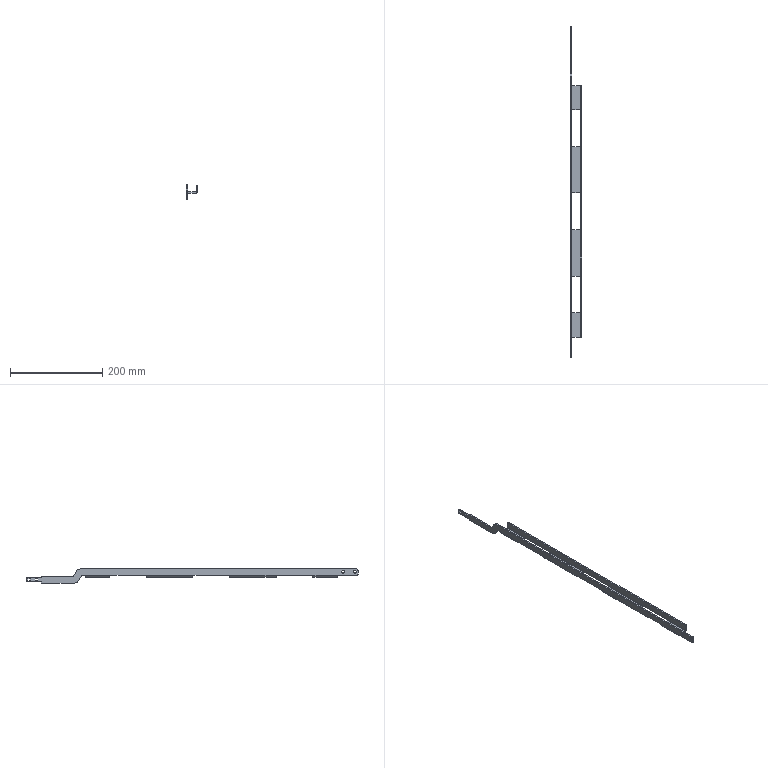Part | SolidWorks | features BaseBody 1 | 1 solid | 85 faces | box 25 x 719 x 30.5 mm | volume 74026 mm3 | plane 57 | cylinder 28 | commonest cylinder face diameters 6 x10 1 x8 7 x8 20 x2